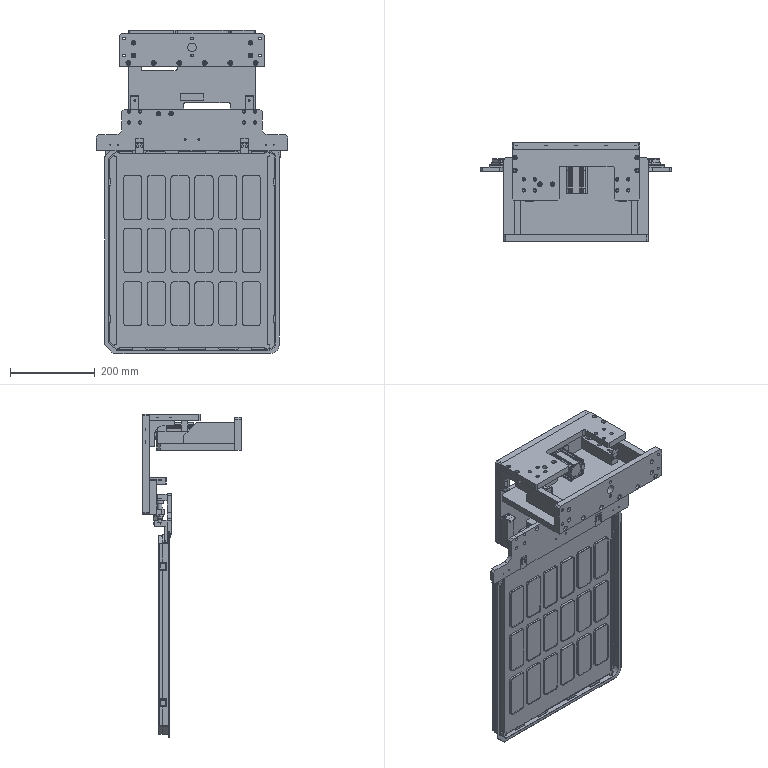Part | NX | 52 solids | 2168 faces | box 450 x 231.5 x 760.75 mm | volume 3988168 mm3 | plane 1153 | cylinder 750 | cone 133 | spline 122 | torus 10 | commonest cylinder face diameters 10 x98 13 x72 3 x66 11 x59 5 x55 6 x43